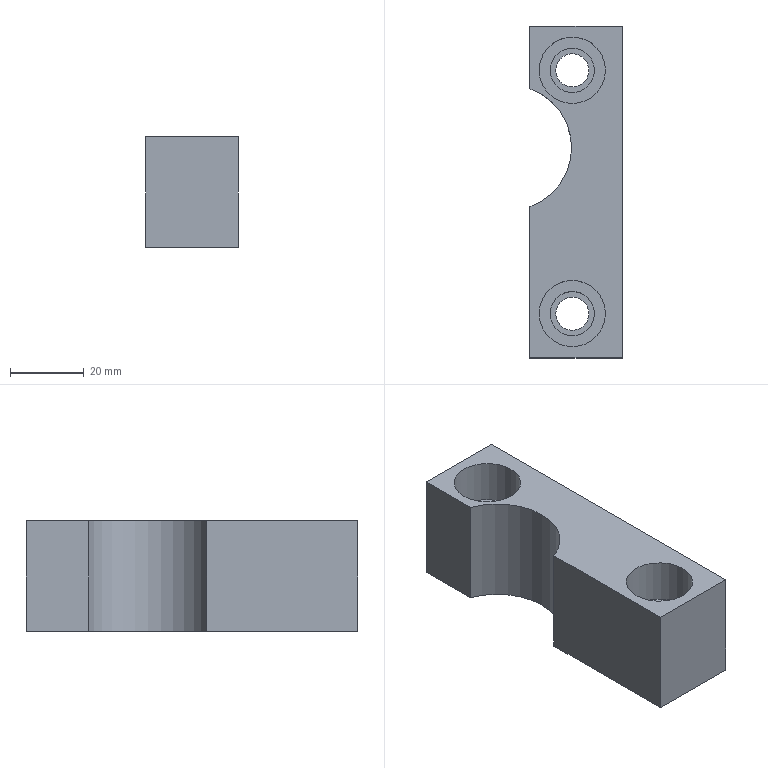Part | STEP file | solid 21 | 1 solid | 18 faces | box 25 x 90 x 30.004 mm | volume 49415 mm3 | plane 11 | cylinder 7 | commonest cylinder face diameters 9 x2 12 x2 18 x2 34 x1